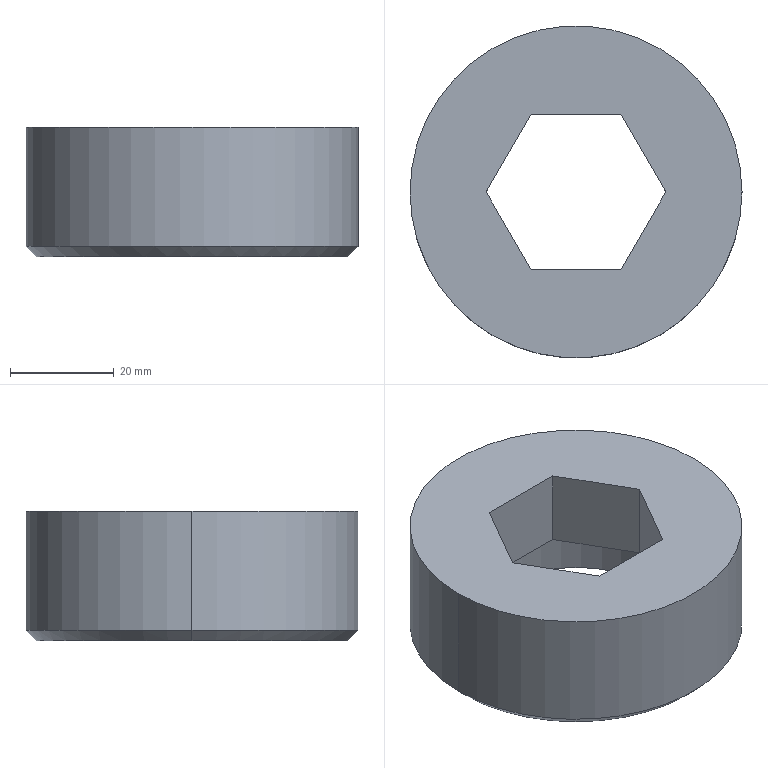Part | SolidWorks | features ICE 2, Chamfer 1, Extrusion 1 | 1 solid | 15 faces | box 64 x 64 x 25 mm | volume 53818 mm3 | plane 9 | cylinder 4 | cone 2 | commonest cylinder face diameters 43 x2 64 x2
STEP:
#1=CARTESIAN_POINT('',(-30.,0.,0.));
#2=VERTEX_POINT('',#1);
#3=CARTESIAN_POINT('',(30.,0.,0.));
#4=VERTEX_POINT('',#3);
#5=CARTESIAN_POINT('',(0.,0.,0.));
#6=DIRECTION('',(0.,0.,-1.));
#7=DIRECTION('',(1.,0.,0.));
#8=AXIS2_PLACEMENT_3D('',#5,#6,#7);
#9=CIRCLE('',#8,30.);
#10=EDGE_CURVE('',#2,#4,#9,.T.);
#11=ORIENTED_EDGE('',*,*,#10,.F.);
#12=CARTESIAN_POINT('',(-32.,0.,2.));
#13=VERTEX_POINT('',#12);
#14=CARTESIAN_POINT('',(-32.,0.,2.));
#15=DIRECTION('',(-0.7071,0.,0.7071));
#16=VECTOR('',#15,1000.);
#17=LINE('',#14,#16);
#18=EDGE_CURVE('',#2,#13,#17,.T.);
#19=ORIENTED_EDGE('',*,*,#18,.T.);
#20=CARTESIAN_POINT('',(32.,0.,2.));
#21=VERTEX_POINT('',#20);
#22=CARTESIAN_POINT('',(0.,0.,2.));
#23=DIRECTION('',(0.,0.,1.));
#24=DIRECTION('',(1.,0.,0.));
#25=AXIS2_PLACEMENT_3D('',#22,#23,#24);
#26=CIRCLE('',#25,32.);
#27=EDGE_CURVE('',#21,#13,#26,.T.);
#28=ORIENTED_EDGE('',*,*,#27,.F.);
#29=CARTESIAN_POINT('',(32.,0.,2.));
#30=DIRECTION('',(0.7071,0.,0.7071));
#31=VECTOR('',#30,1000.);
#32=LINE('',#29,#31);
#33=EDGE_CURVE('',#4,#21,#32,.T.);
#34=ORIENTED_EDGE('',*,*,#33,.F.);
#35=EDGE_LOOP('',(#11,#19,#28,#34));
#36=FACE_OUTER_BOUND('',#35,.T.);
#37=CARTESIAN_POINT('',(0.,0.,2.));
#38=DIRECTION('',(0.,0.,1.));
#39=DIRECTION('',(1.,0.,0.));
#40=AXIS2_PLACEMENT_3D('',#37,#38,#39);
#41=CONICAL_SURFACE('',#40,32.,0.7854);
#42=ADVANCED_FACE('',(#36),#41,.T.);
#43=CARTESIAN_POINT('',(21.5,0.,10.));
#44=VERTEX_POINT('',#43);
#45=CARTESIAN_POINT('',(-21.5,0.,10.));
#46=VERTEX_POINT('',#45);
#47=CARTESIAN_POINT('',(0.,0.,10.));
#48=DIRECTION('',(0.,0.,-1.));
#49=DIRECTION('',(-1.,0.,0.));
#50=AXIS2_PLACEMENT_3D('',#47,#48,#49);
#51=CIRCLE('',#50,21.5);
#52=EDGE_CURVE('',#44,#46,#51,.T.);
#53=ORIENTED_EDGE('',*,*,#52,.F.);
#54=CARTESIAN_POINT('',(21.5,0.,0.));
#55=VERTEX_POINT('',#54);
#56=CARTESIAN_POINT('',(21.5,0.,10.));
#57=DIRECTION('',(0.,0.,-1.));
#58=VECTOR('',#57,1000.);
#59=LINE('',#56,#58);
#60=EDGE_CURVE('',#44,#55,#59,.T.);
#61=ORIENTED_EDGE('',*,*,#60,.T.);
#62=CARTESIAN_POINT('',(-21.5,0.,0.));
#63=VERTEX_POINT('',#62);
#64=CARTESIAN_POINT('',(0.,0.,0.));
#65=DIRECTION('',(0.,0.,-1.));
#66=DIRECTION('',(-1.,0.,0.));
#67=AXIS2_PLACEMENT_3D('',#64,#65,#66);
#68=CIRCLE('',#67,21.5);
#69=EDGE_CURVE('',#55,#63,#68,.T.);
#70=ORIENTED_EDGE('',*,*,#69,.T.);
#71=CARTESIAN_POINT('',(-21.5,0.,10.));
#72=DIRECTION('',(0.,0.,-1.));
#73=VECTOR('',#72,1000.);
#74=LINE('',#71,#73);
#75=EDGE_CURVE('',#46,#63,#74,.T.);
#76=ORIENTED_EDGE('',*,*,#75,.F.);
#77=EDGE_LOOP('',(#53,#61,#70,#76));
#78=FACE_OUTER_BOUND('',#77,.T.);
#79=CARTESIAN_POINT('',(0.,0.,10.));
#80=DIRECTION('',(0.,0.,-1.));
#81=DIRECTION('',(-1.,0.,0.));
#82=AXIS2_PLACEMENT_3D('',#79,#80,#81);
#83=CYLINDRICAL_SURFACE('',#82,21.5);
#84=ADVANCED_FACE('',(#78),#83,.F.);
#85=CARTESIAN_POINT('',(32.,0.,25.));
#86=VERTEX_POINT('',#85);
#87=CARTESIAN_POINT('',(-32.,0.,25.));
#88=VERTEX_POINT('',#87);
#89=CARTESIAN_POINT('',(0.,0.,25.));
#90=DIRECTION('',(0.,0.,1.));
#91=DIRECTION('',(1.,0.,0.));
#92=AXIS2_PLACEMENT_3D('',#89,#90,#91);
#93=CIRCLE('',#92,32.);
#94=EDGE_CURVE('',#86,#88,#93,.T.);
#95=ORIENTED_EDGE('',*,*,#94,.F.);
#96=CARTESIAN_POINT('',(32.,0.,25.));
#97=DIRECTION('',(0.,0.,-1.));
#98=VECTOR('',#97,1000.);
#99=LINE('',#96,#98);
#100=EDGE_CURVE('',#86,#21,#99,.T.);
#101=ORIENTED_EDGE('',*,*,#100,.T.);
#102=ORIENTED_EDGE('',*,*,#27,.T.);
#103=CARTESIAN_POINT('',(-32.,0.,25.));
#104=DIRECTION('',(0.,0.,-1.));
#105=VECTOR('',#104,1000.);
#106=LINE('',#103,#105);
#107=EDGE_CURVE('',#88,#13,#106,.T.);
#108=ORIENTED_EDGE('',*,*,#107,.F.);
#109=EDGE_LOOP('',(#95,#101,#102,#108));
#110=FACE_OUTER_BOUND('',#109,.T.);
#111=CARTESIAN_POINT('',(0.,0.,25.));
#112=DIRECTION('',(0.,0.,-1.));
#113=DIRECTION('',(-1.,0.,0.));
#114=AXIS2_PLACEMENT_3D('',#111,#112,#113);
#115=CYLINDRICAL_SURFACE('',#114,32.);
#116=ADVANCED_FACE('',(#110),#115,.T.);
#117=CARTESIAN_POINT('',(8.66,-15.,10.));
#118=VERTEX_POINT('',#117);
#119=CARTESIAN_POINT('',(17.321,0.,10.));
#120=VERTEX_POINT('',#119);
#121=CARTESIAN_POINT('',(8.66,-15.,10.));
#122=DIRECTION('',(0.5,0.866,0.));
#123=VECTOR('',#122,1000.);
#124=LINE('',#121,#123);
#125=EDGE_CURVE('',#118,#120,#124,.T.);
#126=ORIENTED_EDGE('',*,*,#125,.F.);
#127=CARTESIAN_POINT('',(8.66,-15.,25.));
#128=VERTEX_POINT('',#127);
#129=CARTESIAN_POINT('',(8.66,-15.,0.));
#130=DIRECTION('',(0.,0.,1.));
#131=VECTOR('',#130,1000.);
#132=LINE('',#129,#131);
#133=EDGE_CURVE('',#118,#128,#132,.T.);
#134=ORIENTED_EDGE('',*,*,#133,.T.);
#135=CARTESIAN_POINT('',(17.321,0.,25.));
#136=VERTEX_POINT('',#135);
#137=CARTESIAN_POINT('',(8.66,-15.,25.));
#138=DIRECTION('',(0.5,0.866,0.));
#139=VECTOR('',#138,1000.);
#140=LINE('',#137,#139);
#141=EDGE_CURVE('',#128,#136,#140,.T.);
#142=ORIENTED_EDGE('',*,*,#141,.T.);
#143=CARTESIAN_POINT('',(17.321,0.,0.));
#144=DIRECTION('',(0.,0.,1.));
#145=VECTOR('',#144,1000.);
#146=LINE('',#143,#145);
#147=EDGE_CURVE('',#120,#136,#146,.T.);
#148=ORIENTED_EDGE('',*,*,#147,.F.);
#149=EDGE_LOOP('',(#126,#134,#142,#148));
#150=FACE_OUTER_BOUND('',#149,.T.);
#151=CARTESIAN_POINT('',(8.66,-15.,0.));
#152=DIRECTION('',(0.866,-0.5,0.));
#153=DIRECTION('',(0.5,0.866,0.));
#154=AXIS2_PLACEMENT_3D('',#151,#152,#153);
#155=PLANE('',#154);
#156=ADVANCED_FACE('',(#150),#155,.F.);
#157=CARTESIAN_POINT('',(-8.66,-15.,10.));
#158=VERTEX_POINT('',#157);
#159=CARTESIAN_POINT('',(-8.66,-15.,10.));
#160=DIRECTION('',(1.,0.,0.));
#161=VECTOR('',#160,1000.);
#162=LINE('',#159,#161);
#163=EDGE_CURVE('',#158,#118,#162,.T.);
#164=ORIENTED_EDGE('',*,*,#163,.F.);
#165=CARTESIAN_POINT('',(-8.66,-15.,25.));
#166=VERTEX_POINT('',#165);
#167=CARTESIAN_POINT('',(-8.66,-15.,0.));
#168=DIRECTION('',(0.,0.,1.));
#169=VECTOR('',#168,1000.);
#170=LINE('',#167,#169);
#171=EDGE_CURVE('',#158,#166,#170,.T.);
#172=ORIENTED_EDGE('',*,*,#171,.T.);
#173=CARTESIAN_POINT('',(-8.66,-15.,25.));
#174=DIRECTION('',(1.,0.,0.));
#175=VECTOR('',#174,1000.);
#176=LINE('',#173,#175);
#177=EDGE_CURVE('',#166,#128,#176,.T.);
#178=ORIENTED_EDGE('',*,*,#177,.T.);
#179=ORIENTED_EDGE('',*,*,#133,.F.);
#180=EDGE_LOOP('',(#164,#172,#178,#179));
#181=FACE_OUTER_BOUND('',#180,.T.);
#182=CARTESIAN_POINT('',(-8.66,-15.,0.));
#183=DIRECTION('',(0.,-1.,0.));
#184=DIRECTION('',(1.,0.,0.));
#185=AXIS2_PLACEMENT_3D('',#182,#183,#184);
#186=PLANE('',#185);
#187=ADVANCED_FACE('',(#181),#186,.F.);
#188=CARTESIAN_POINT('',(-17.321,0.,10.));
#189=VERTEX_POINT('',#188);
#190=CARTESIAN_POINT('',(-17.321,0.,10.));
#191=DIRECTION('',(0.5,-0.866,0.));
#192=VECTOR('',#191,1000.);
#193=LINE('',#190,#192);
#194=EDGE_CURVE('',#189,#158,#193,.T.);
#195=ORIENTED_EDGE('',*,*,#194,.F.);
#196=CARTESIAN_POINT('',(-17.321,0.,25.));
#197=VERTEX_POINT('',#196);
#198=CARTESIAN_POINT('',(-17.321,0.,0.));
#199=DIRECTION('',(0.,0.,1.));
#200=VECTOR('',#199,1000.);
#201=LINE('',#198,#200);
#202=EDGE_CURVE('',#189,#197,#201,.T.);
#203=ORIENTED_EDGE('',*,*,#202,.T.);
#204=CARTESIAN_POINT('',(-17.321,0.,25.));
#205=DIRECTION('',(0.5,-0.866,0.));
#206=VECTOR('',#205,1000.);
#207=LINE('',#204,#206);
#208=EDGE_CURVE('',#197,#166,#207,.T.);
#209=ORIENTED_EDGE('',*,*,#208,.T.);
#210=ORIENTED_EDGE('',*,*,#171,.F.);
#211=EDGE_LOOP('',(#195,#203,#209,#210));
#212=FACE_OUTER_BOUND('',#211,.T.);
#213=CARTESIAN_POINT('',(-17.321,0.,0.));
#214=DIRECTION('',(-0.866,-0.5,0.));
#215=DIRECTION('',(0.5,-0.866,0.));
#216=AXIS2_PLACEMENT_3D('',#213,#214,#215);
#217=PLANE('',#216);
#218=ADVANCED_FACE('',(#212),#217,.F.);
#219=CARTESIAN_POINT('',(-8.66,15.,10.));
#220=VERTEX_POINT('',#219);
#221=CARTESIAN_POINT('',(-8.66,15.,10.));
#222=DIRECTION('',(-0.5,-0.866,0.));
#223=VECTOR('',#222,1000.);
#224=LINE('',#221,#223);
#225=EDGE_CURVE('',#220,#189,#224,.T.);
#226=ORIENTED_EDGE('',*,*,#225,.F.);
#227=CARTESIAN_POINT('',(-8.66,15.,25.));
#228=VERTEX_POINT('',#227);
#229=CARTESIAN_POINT('',(-8.66,15.,0.));
#230=DIRECTION('',(0.,0.,1.));
#231=VECTOR('',#230,1000.);
#232=LINE('',#229,#231);
#233=EDGE_CURVE('',#220,#228,#232,.T.);
#234=ORIENTED_EDGE('',*,*,#233,.T.);
#235=CARTESIAN_POINT('',(-8.66,15.,25.));
#236=DIRECTION('',(-0.5,-0.866,0.));
#237=VECTOR('',#236,1000.);
#238=LINE('',#235,#237);
#239=EDGE_CURVE('',#228,#197,#238,.T.);
#240=ORIENTED_EDGE('',*,*,#239,.T.);
#241=ORIENTED_EDGE('',*,*,#202,.F.);
#242=EDGE_LOOP('',(#226,#234,#240,#241));
#243=FACE_OUTER_BOUND('',#242,.T.);
#244=CARTESIAN_POINT('',(-8.66,15.,0.));
#245=DIRECTION('',(-0.866,0.5,0.));
#246=DIRECTION('',(-0.5,-0.866,0.));
#247=AXIS2_PLACEMENT_3D('',#244,#245,#246);
#248=PLANE('',#247);
#249=ADVANCED_FACE('',(#243),#248,.F.);
#250=CARTESIAN_POINT('',(8.66,15.,10.));
#251=VERTEX_POINT('',#250);
#252=CARTESIAN_POINT('',(8.66,15.,10.));
#253=DIRECTION('',(-1.,0.,0.));
#254=VECTOR('',#253,1000.);
#255=LINE('',#252,#254);
#256=EDGE_CURVE('',#251,#220,#255,.T.);
#257=ORIENTED_EDGE('',*,*,#256,.F.);
#258=CARTESIAN_POINT('',(8.66,15.,25.));
#259=VERTEX_POINT('',#258);
#260=CARTESIAN_POINT('',(8.66,15.,0.));
#261=DIRECTION('',(0.,0.,1.));
#262=VECTOR('',#261,1000.);
#263=LINE('',#260,#262);
#264=EDGE_CURVE('',#251,#259,#263,.T.);
#265=ORIENTED_EDGE('',*,*,#264,.T.);
#266=CARTESIAN_POINT('',(8.66,15.,25.));
#267=DIRECTION('',(-1.,0.,0.));
#268=VECTOR('',#267,1000.);
#269=LINE('',#266,#268);
#270=EDGE_CURVE('',#259,#228,#269,.T.);
#271=ORIENTED_EDGE('',*,*,#270,.T.);
#272=ORIENTED_EDGE('',*,*,#233,.F.);
#273=EDGE_LOOP('',(#257,#265,#271,#272));
#274=FACE_OUTER_BOUND('',#273,.T.);
#275=CARTESIAN_POINT('',(8.66,15.,0.));
#276=DIRECTION('',(0.,1.,0.));
#277=DIRECTION('',(-1.,0.,0.));
#278=AXIS2_PLACEMENT_3D('',#275,#276,#277);
#279=PLANE('',#278);
#280=ADVANCED_FACE('',(#274),#279,.F.);
#281=CARTESIAN_POINT('',(17.321,0.,10.));
#282=DIRECTION('',(-0.5,0.866,0.));
#283=VECTOR('',#282,1000.);
#284=LINE('',#281,#283);
#285=EDGE_CURVE('',#120,#251,#284,.T.);
#286=ORIENTED_EDGE('',*,*,#285,.F.);
#287=ORIENTED_EDGE('',*,*,#147,.T.);
#288=CARTESIAN_POINT('',(17.321,0.,25.));
#289=DIRECTION('',(-0.5,0.866,0.));
#290=VECTOR('',#289,1000.);
#291=LINE('',#288,#290);
#292=EDGE_CURVE('',#136,#259,#291,.T.);
#293=ORIENTED_EDGE('',*,*,#292,.T.);
#294=ORIENTED_EDGE('',*,*,#264,.F.);
#295=EDGE_LOOP('',(#286,#287,#293,#294));
#296=FACE_OUTER_BOUND('',#295,.T.);
#297=CARTESIAN_POINT('',(17.321,0.,0.));
#298=DIRECTION('',(0.866,0.5,0.));
#299=DIRECTION('',(-0.5,0.866,0.));
#300=AXIS2_PLACEMENT_3D('',#297,#298,#299);
#301=PLANE('',#300);
#302=ADVANCED_FACE('',(#296),#301,.F.);
#303=ORIENTED_EDGE('',*,*,#100,.F.);
#304=CARTESIAN_POINT('',(0.,0.,25.));
#305=DIRECTION('',(0.,0.,1.));
#306=DIRECTION('',(1.,0.,0.));
#307=AXIS2_PLACEMENT_3D('',#304,#305,#306);
#308=CIRCLE('',#307,32.);
#309=EDGE_CURVE('',#88,#86,#308,.T.);
#310=ORIENTED_EDGE('',*,*,#309,.F.);
#311=ORIENTED_EDGE('',*,*,#107,.T.);
#312=CARTESIAN_POINT('',(0.,0.,2.));
#313=DIRECTION('',(0.,0.,1.));
#314=DIRECTION('',(1.,0.,0.));
#315=AXIS2_PLACEMENT_3D('',#312,#313,#314);
#316=CIRCLE('',#315,32.);
#317=EDGE_CURVE('',#13,#21,#316,.T.);
#318=ORIENTED_EDGE('',*,*,#317,.T.);
#319=EDGE_LOOP('',(#303,#310,#311,#318));
#320=FACE_OUTER_BOUND('',#319,.T.);
#321=CARTESIAN_POINT('',(0.,0.,25.));
#322=DIRECTION('',(0.,0.,-1.));
#323=DIRECTION('',(-1.,0.,0.));
#324=AXIS2_PLACEMENT_3D('',#321,#322,#323);
#325=CYLINDRICAL_SURFACE('',#324,32.);
#326=ADVANCED_FACE('',(#320),#325,.T.);
#327=ORIENTED_EDGE('',*,*,#141,.F.);
#328=ORIENTED_EDGE('',*,*,#177,.F.);
#329=ORIENTED_EDGE('',*,*,#208,.F.);
#330=ORIENTED_EDGE('',*,*,#239,.F.);
#331=ORIENTED_EDGE('',*,*,#270,.F.);
#332=ORIENTED_EDGE('',*,*,#292,.F.);
#333=EDGE_LOOP('',(#327,#328,#329,#330,#331,#332));
#334=FACE_BOUND('',#333,.T.);
#335=ORIENTED_EDGE('',*,*,#309,.T.);
#336=ORIENTED_EDGE('',*,*,#94,.T.);
#337=EDGE_LOOP('',(#335,#336));
#338=FACE_OUTER_BOUND('',#337,.T.);
#339=CARTESIAN_POINT('',(0.,0.,25.));
#340=DIRECTION('',(0.,0.,1.));
#341=DIRECTION('',(1.,0.,0.));
#342=AXIS2_PLACEMENT_3D('',#339,#340,#341);
#343=PLANE('',#342);
#344=ADVANCED_FACE('',(#334,#338),#343,.T.);
#345=CARTESIAN_POINT('',(0.,0.,0.));
#346=DIRECTION('',(0.,0.,-1.));
#347=DIRECTION('',(1.,0.,0.));
#348=AXIS2_PLACEMENT_3D('',#345,#346,#347);
#349=CIRCLE('',#348,30.);
#350=EDGE_CURVE('',#4,#2,#349,.T.);
#351=ORIENTED_EDGE('',*,*,#350,.T.);
#352=ORIENTED_EDGE('',*,*,#10,.T.);
#353=EDGE_LOOP('',(#351,#352));
#354=FACE_OUTER_BOUND('',#353,.T.);
#355=CARTESIAN_POINT('',(0.,0.,0.));
#356=DIRECTION('',(0.,0.,-1.));
#357=DIRECTION('',(-1.,0.,0.));
#358=AXIS2_PLACEMENT_3D('',#355,#356,#357);
#359=CIRCLE('',#358,21.5);
#360=EDGE_CURVE('',#63,#55,#359,.T.);
#361=ORIENTED_EDGE('',*,*,#360,.F.);
#362=ORIENTED_EDGE('',*,*,#69,.F.);
#363=EDGE_LOOP('',(#361,#362));
#364=FACE_BOUND('',#363,.T.);
#365=CARTESIAN_POINT('',(0.,0.,0.));
#366=DIRECTION('',(0.,0.,1.));
#367=DIRECTION('',(1.,0.,0.));
#368=AXIS2_PLACEMENT_3D('',#365,#366,#367);
#369=PLANE('',#368);
#370=ADVANCED_FACE('',(#354,#364),#369,.F.);
#371=CARTESIAN_POINT('',(0.,0.,10.));
#372=DIRECTION('',(0.,0.,-1.));
#373=DIRECTION('',(-1.,0.,0.));
#374=AXIS2_PLACEMENT_3D('',#371,#372,#373);
#375=CIRCLE('',#374,21.5);
#376=EDGE_CURVE('',#46,#44,#375,.T.);
#377=ORIENTED_EDGE('',*,*,#376,.T.);
#378=ORIENTED_EDGE('',*,*,#52,.T.);
#379=EDGE_LOOP('',(#377,#378));
#380=FACE_OUTER_BOUND('',#379,.T.);
#381=ORIENTED_EDGE('',*,*,#125,.T.);
#382=ORIENTED_EDGE('',*,*,#285,.T.);
#383=ORIENTED_EDGE('',*,*,#256,.T.);
#384=ORIENTED_EDGE('',*,*,#225,.T.);
#385=ORIENTED_EDGE('',*,*,#194,.T.);
#386=ORIENTED_EDGE('',*,*,#163,.T.);
#387=EDGE_LOOP('',(#381,#382,#383,#384,#385,#386));
#388=FACE_BOUND('',#387,.T.);
#389=CARTESIAN_POINT('',(0.,0.,10.));
#390=DIRECTION('',(0.,0.,-1.));
#391=DIRECTION('',(-1.,0.,0.));
#392=AXIS2_PLACEMENT_3D('',#389,#390,#391);
#393=PLANE('',#392);
#394=ADVANCED_FACE('',(#380,#388),#393,.T.);
#395=ORIENTED_EDGE('',*,*,#60,.F.);
#396=ORIENTED_EDGE('',*,*,#376,.F.);
#397=ORIENTED_EDGE('',*,*,#75,.T.);
#398=ORIENTED_EDGE('',*,*,#360,.T.);
#399=EDGE_LOOP('',(#395,#396,#397,#398));
#400=FACE_OUTER_BOUND('',#399,.T.);
#401=CARTESIAN_POINT('',(0.,0.,10.));
#402=DIRECTION('',(0.,0.,-1.));
#403=DIRECTION('',(-1.,0.,0.));
#404=AXIS2_PLACEMENT_3D('',#401,#402,#403);
#405=CYLINDRICAL_SURFACE('',#404,21.5);
#406=ADVANCED_FACE('',(#400),#405,.F.);
#407=ORIENTED_EDGE('',*,*,#18,.F.);
#408=ORIENTED_EDGE('',*,*,#350,.F.);
#409=ORIENTED_EDGE('',*,*,#33,.T.);
#410=ORIENTED_EDGE('',*,*,#317,.F.);
#411=EDGE_LOOP('',(#407,#408,#409,#410));
#412=FACE_OUTER_BOUND('',#411,.T.);
#413=CARTESIAN_POINT('',(0.,0.,2.));
#414=DIRECTION('',(0.,0.,1.));
#415=DIRECTION('',(1.,0.,0.));
#416=AXIS2_PLACEMENT_3D('',#413,#414,#415);
#417=CONICAL_SURFACE('',#416,32.,0.7854);
#418=ADVANCED_FACE('',(#412),#417,.T.);
#419=CLOSED_SHELL('',(#42,#84,#116,#156,#187,#218,#249,#280,#302,#326,#344,#370,#394,#406,#418));
#420=MANIFOLD_SOLID_BREP('',#419);
#421=CARTESIAN_POINT('',(0.,0.,0.));
#422=DIRECTION('',(0.,0.,1.));
#423=DIRECTION('',(1.,0.,0.));
#424=AXIS2_PLACEMENT_3D('',#421,#422,#423);
#425=(LENGTH_UNIT()NAMED_UNIT(*)SI_UNIT(.MILLI.,.METRE.));
#426=UNCERTAINTY_MEASURE_WITH_UNIT(LENGTH_MEASURE(0.00001),#425,'','');
#427=(NAMED_UNIT(*)PLANE_ANGLE_UNIT()SI_UNIT($,.RADIAN.));
#428=(NAMED_UNIT(*)SI_UNIT($,.STERADIAN.)SOLID_ANGLE_UNIT());
#429=(GEOMETRIC_REPRESENTATION_CONTEXT(3)GLOBAL_UNCERTAINTY_ASSIGNED_CONTEXT((#426))GLOBAL_UNIT_ASSIGNED_CONTEXT((#425,#427,#428))REPRESENTATION_CONTEXT('',''));
#430=ADVANCED_BREP_SHAPE_REPRESENTATION('',(#420,#424),#429);